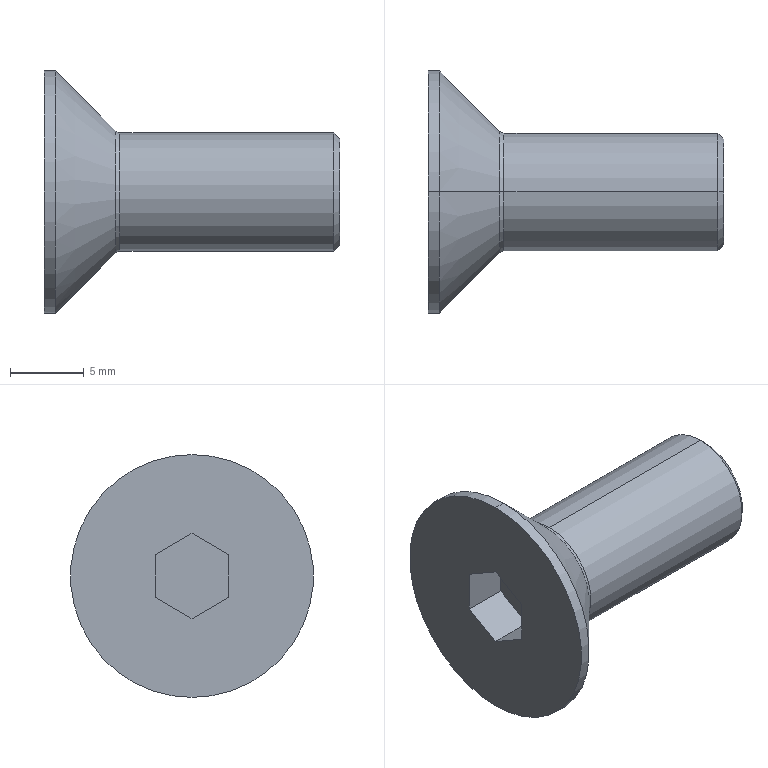Part | STEP file | 1 solid | 19 faces | box 20 x 16.428 x 16.428 mm | volume 1361 mm3 | plane 9 | cone 4 | cylinder 4 | spline 2 | commonest cylinder face diameters 8 x2 16.428 x2
STEP:
#1=CARTESIAN_POINT('',(0.,0.,0.));
#2=DIRECTION('',(0.,0.,1.));
#3=DIRECTION('',(1.,0.,0.));
#4=AXIS2_PLACEMENT_3D('',#1,#2,#3);
#5=CARTESIAN_POINT('',(15.04,0.,3.6));
#6=VERTEX_POINT('',#5);
#7=CARTESIAN_POINT('',(15.04,0.,-3.6));
#8=VERTEX_POINT('',#7);
#9=CARTESIAN_POINT('',(15.04,0.,0.));
#10=DIRECTION('',(-1.,0.,0.));
#11=DIRECTION('',(0.,0.,1.));
#12=AXIS2_PLACEMENT_3D('',#9,#10,#11);
#13=CIRCLE('',#12,3.6);
#14=CARTESIAN_POINT('',(15.04,4.,0.));
#15=DIRECTION('',(-1.,0.,0.));
#16=DIRECTION('',(0.,0.,1.));
#17=AXIS2_PLACEMENT_3D('',#14,#15,#16);
#18=PLANE('',#17);
#19=CARTESIAN_POINT('',(0.,-4.));
#20=DIRECTION('',(1.,0.));
#21=AXIS2_PLACEMENT_2D('',#19,#20);
#22=CIRCLE('',#21,3.6);
#23=(GEOMETRIC_REPRESENTATION_CONTEXT(2)PARAMETRIC_REPRESENTATION_CONTEXT()REPRESENTATION_CONTEXT('',''));
#24=DEFINITIONAL_REPRESENTATION('',(#22),#23);
#25=PCURVE('',#18,#24);
#26=CARTESIAN_POINT('',(14.64,0.,0.));
#27=DIRECTION('',(-1.,0.,0.));
#28=DIRECTION('',(0.,0.,1.));
#29=AXIS2_PLACEMENT_3D('',#26,#27,#28);
#30=CONICAL_SURFACE('',#29,4.,0.7854);
#31=CARTESIAN_POINT('',(0.,-0.4));
#32=DIRECTION('',(1.,0.));
#33=VECTOR('',#32,1.);
#34=LINE('',#31,#33);
#35=(GEOMETRIC_REPRESENTATION_CONTEXT(2)PARAMETRIC_REPRESENTATION_CONTEXT()REPRESENTATION_CONTEXT('',''));
#36=DEFINITIONAL_REPRESENTATION('',(#34),#35);
#37=PCURVE('',#30,#36);
#38=SURFACE_CURVE('',#13,(#25,#37),.PCURVE_S1.);
#39=EDGE_CURVE('',#6,#8,#38,.T.);
#40=ORIENTED_EDGE('',*,*,#39,.F.);
#41=CARTESIAN_POINT('',(15.04,0.,0.));
#42=DIRECTION('',(-1.,0.,0.));
#43=DIRECTION('',(0.,0.,1.));
#44=AXIS2_PLACEMENT_3D('',#41,#42,#43);
#45=CIRCLE('',#44,3.6);
#46=CARTESIAN_POINT('',(0.,-4.));
#47=DIRECTION('',(1.,0.));
#48=AXIS2_PLACEMENT_2D('',#46,#47);
#49=CIRCLE('',#48,3.6);
#50=(GEOMETRIC_REPRESENTATION_CONTEXT(2)PARAMETRIC_REPRESENTATION_CONTEXT()REPRESENTATION_CONTEXT('',''));
#51=DEFINITIONAL_REPRESENTATION('',(#49),#50);
#52=PCURVE('',#18,#51);
#53=CARTESIAN_POINT('',(14.64,0.,0.));
#54=DIRECTION('',(-1.,0.,0.));
#55=DIRECTION('',(0.,0.,1.));
#56=AXIS2_PLACEMENT_3D('',#53,#54,#55);
#57=CONICAL_SURFACE('',#56,4.,0.7854);
#58=CARTESIAN_POINT('',(0.,-0.4));
#59=DIRECTION('',(1.,0.));
#60=VECTOR('',#59,1.);
#61=LINE('',#58,#60);
#62=(GEOMETRIC_REPRESENTATION_CONTEXT(2)PARAMETRIC_REPRESENTATION_CONTEXT()REPRESENTATION_CONTEXT('',''));
#63=DEFINITIONAL_REPRESENTATION('',(#61),#62);
#64=PCURVE('',#57,#63);
#65=SURFACE_CURVE('',#45,(#52,#64),.PCURVE_S1.);
#66=EDGE_CURVE('',#8,#6,#65,.T.);
#67=ORIENTED_EDGE('',*,*,#66,.F.);
#68=EDGE_LOOP('',(#40,#67));
#69=FACE_BOUND('',#68,.T.);
#70=ADVANCED_FACE('',(#69),#18,.F.);
#71=CARTESIAN_POINT('',(14.64,0.,-4.));
#72=VERTEX_POINT('',#71);
#73=CARTESIAN_POINT('',(14.64,0.,-4.));
#74=DIRECTION('',(-0.7071,0.,-0.7071));
#75=VECTOR('',#74,1.);
#76=LINE('',#73,#75);
#77=CARTESIAN_POINT('',(3.142,0.));
#78=DIRECTION('',(0.,1.));
#79=VECTOR('',#78,1.);
#80=LINE('',#77,#79);
#81=(GEOMETRIC_REPRESENTATION_CONTEXT(2)PARAMETRIC_REPRESENTATION_CONTEXT()REPRESENTATION_CONTEXT('',''));
#82=DEFINITIONAL_REPRESENTATION('',(#80),#81);
#83=PCURVE('',#57,#82);
#84=CARTESIAN_POINT('',(3.142,0.));
#85=DIRECTION('',(0.,1.));
#86=VECTOR('',#85,1.);
#87=LINE('',#84,#86);
#88=(GEOMETRIC_REPRESENTATION_CONTEXT(2)PARAMETRIC_REPRESENTATION_CONTEXT()REPRESENTATION_CONTEXT('',''));
#89=DEFINITIONAL_REPRESENTATION('',(#87),#88);
#90=PCURVE('',#30,#89);
#91=SURFACE_CURVE('',#76,(#83,#90),.PCURVE_S1.);
#92=EDGE_CURVE('',#8,#72,#91,.T.);
#93=ORIENTED_EDGE('',*,*,#92,.F.);
#94=ORIENTED_EDGE('',*,*,#66,.T.);
#95=CARTESIAN_POINT('',(14.64,0.,4.));
#96=VERTEX_POINT('',#95);
#97=CARTESIAN_POINT('',(14.64,0.,4.));
#98=DIRECTION('',(-0.7071,0.,0.7071));
#99=VECTOR('',#98,1.);
#100=LINE('',#97,#99);
#101=CARTESIAN_POINT('',(6.283,0.));
#102=DIRECTION('',(0.,1.));
#103=VECTOR('',#102,1.);
#104=LINE('',#101,#103);
#105=(GEOMETRIC_REPRESENTATION_CONTEXT(2)PARAMETRIC_REPRESENTATION_CONTEXT()REPRESENTATION_CONTEXT('',''));
#106=DEFINITIONAL_REPRESENTATION('',(#104),#105);
#107=PCURVE('',#57,#106);
#108=CARTESIAN_POINT('',(0.,0.));
#109=DIRECTION('',(0.,1.));
#110=VECTOR('',#109,1.);
#111=LINE('',#108,#110);
#112=(GEOMETRIC_REPRESENTATION_CONTEXT(2)PARAMETRIC_REPRESENTATION_CONTEXT()REPRESENTATION_CONTEXT('',''));
#113=DEFINITIONAL_REPRESENTATION('',(#111),#112);
#114=PCURVE('',#30,#113);
#115=SURFACE_CURVE('',#100,(#107,#114),.PCURVE_S1.);
#116=EDGE_CURVE('',#6,#96,#115,.T.);
#117=ORIENTED_EDGE('',*,*,#116,.T.);
#118=CARTESIAN_POINT('',(14.64,0.,0.));
#119=DIRECTION('',(-1.,0.,0.));
#120=DIRECTION('',(0.,0.,1.));
#121=AXIS2_PLACEMENT_3D('',#118,#119,#120);
#122=CIRCLE('',#121,4.);
#123=CARTESIAN_POINT('',(0.,0.));
#124=DIRECTION('',(1.,0.));
#125=VECTOR('',#124,1.);
#126=LINE('',#123,#125);
#127=(GEOMETRIC_REPRESENTATION_CONTEXT(2)PARAMETRIC_REPRESENTATION_CONTEXT()REPRESENTATION_CONTEXT('',''));
#128=DEFINITIONAL_REPRESENTATION('',(#126),#127);
#129=PCURVE('',#57,#128);
#130=CARTESIAN_POINT('',(-23.423,0.,0.));
#131=DIRECTION('',(-1.,0.,0.));
#132=DIRECTION('',(0.,0.,1.));
#133=AXIS2_PLACEMENT_3D('',#130,#131,#132);
#134=CYLINDRICAL_SURFACE('',#133,4.);
#135=CARTESIAN_POINT('',(0.,-38.063));
#136=DIRECTION('',(1.,0.));
#137=VECTOR('',#136,1.);
#138=LINE('',#135,#137);
#139=(GEOMETRIC_REPRESENTATION_CONTEXT(2)PARAMETRIC_REPRESENTATION_CONTEXT()REPRESENTATION_CONTEXT('',''));
#140=DEFINITIONAL_REPRESENTATION('',(#138),#139);
#141=PCURVE('',#134,#140);
#142=SURFACE_CURVE('',#122,(#129,#141),.PCURVE_S1.);
#143=EDGE_CURVE('',#72,#96,#142,.T.);
#144=ORIENTED_EDGE('',*,*,#143,.F.);
#145=EDGE_LOOP('',(#93,#94,#117,#144));
#146=FACE_BOUND('',#145,.T.);
#147=ADVANCED_FACE('',(#146),#57,.T.);
#148=CARTESIAN_POINT('',(0.1657,0.,-4.));
#149=VERTEX_POINT('',#148);
#150=CARTESIAN_POINT('',(-23.423,0.,-4.));
#151=DIRECTION('',(-1.,0.,0.));
#152=VECTOR('',#151,1.);
#153=LINE('',#150,#152);
#154=CARTESIAN_POINT('',(3.142,0.));
#155=DIRECTION('',(0.,1.));
#156=VECTOR('',#155,1.);
#157=LINE('',#154,#156);
#158=(GEOMETRIC_REPRESENTATION_CONTEXT(2)PARAMETRIC_REPRESENTATION_CONTEXT()REPRESENTATION_CONTEXT('',''));
#159=DEFINITIONAL_REPRESENTATION('',(#157),#158);
#160=PCURVE('',#134,#159);
#161=CARTESIAN_POINT('',(-23.423,0.,0.));
#162=DIRECTION('',(-1.,0.,0.));
#163=DIRECTION('',(0.,0.,1.));
#164=AXIS2_PLACEMENT_3D('',#161,#162,#163);
#165=CYLINDRICAL_SURFACE('',#164,4.);
#166=CARTESIAN_POINT('',(3.142,0.));
#167=DIRECTION('',(0.,1.));
#168=VECTOR('',#167,1.);
#169=LINE('',#166,#168);
#170=(GEOMETRIC_REPRESENTATION_CONTEXT(2)PARAMETRIC_REPRESENTATION_CONTEXT()REPRESENTATION_CONTEXT('',''));
#171=DEFINITIONAL_REPRESENTATION('',(#169),#170);
#172=PCURVE('',#165,#171);
#173=SURFACE_CURVE('',#153,(#160,#172),.PCURVE_S1.);
#174=EDGE_CURVE('',#72,#149,#173,.T.);
#175=ORIENTED_EDGE('',*,*,#174,.F.);
#176=ORIENTED_EDGE('',*,*,#143,.T.);
#177=CARTESIAN_POINT('',(0.1657,0.,4.));
#178=VERTEX_POINT('',#177);
#179=CARTESIAN_POINT('',(-23.423,0.,4.));
#180=DIRECTION('',(-1.,0.,0.));
#181=VECTOR('',#180,1.);
#182=LINE('',#179,#181);
#183=CARTESIAN_POINT('',(6.283,0.));
#184=DIRECTION('',(0.,1.));
#185=VECTOR('',#184,1.);
#186=LINE('',#183,#185);
#187=(GEOMETRIC_REPRESENTATION_CONTEXT(2)PARAMETRIC_REPRESENTATION_CONTEXT()REPRESENTATION_CONTEXT('',''));
#188=DEFINITIONAL_REPRESENTATION('',(#186),#187);
#189=PCURVE('',#134,#188);
#190=CARTESIAN_POINT('',(0.,0.));
#191=DIRECTION('',(0.,1.));
#192=VECTOR('',#191,1.);
#193=LINE('',#190,#192);
#194=(GEOMETRIC_REPRESENTATION_CONTEXT(2)PARAMETRIC_REPRESENTATION_CONTEXT()REPRESENTATION_CONTEXT('',''));
#195=DEFINITIONAL_REPRESENTATION('',(#193),#194);
#196=PCURVE('',#165,#195);
#197=SURFACE_CURVE('',#182,(#189,#196),.PCURVE_S1.);
#198=EDGE_CURVE('',#96,#178,#197,.T.);
#199=ORIENTED_EDGE('',*,*,#198,.T.);
#200=CARTESIAN_POINT('',(0.1657,0.,0.));
#201=DIRECTION('',(1.,0.,0.));
#202=DIRECTION('',(0.,0.,1.));
#203=AXIS2_PLACEMENT_3D('',#200,#201,#202);
#204=CIRCLE('',#203,4.);
#205=CARTESIAN_POINT('',(6.283,-23.589));
#206=DIRECTION('',(-1.,0.));
#207=VECTOR('',#206,1.);
#208=LINE('',#205,#207);
#209=(GEOMETRIC_REPRESENTATION_CONTEXT(2)PARAMETRIC_REPRESENTATION_CONTEXT()REPRESENTATION_CONTEXT('',''));
#210=DEFINITIONAL_REPRESENTATION('',(#208),#209);
#211=PCURVE('',#134,#210);
#212=CARTESIAN_POINT('',(0.1657,0.,-4.));
#213=CARTESIAN_POINT('',(0.1657,-8.,-4.));
#214=CARTESIAN_POINT('',(0.1657,-8.,4.));
#215=CARTESIAN_POINT('',(0.1657,0.,4.));
#216=CARTESIAN_POINT('',(0.05818,0.,-4.));
#217=CARTESIAN_POINT('',(0.05818,-8.,-4.));
#218=CARTESIAN_POINT('',(0.05818,-8.,4.));
#219=CARTESIAN_POINT('',(0.05818,0.,4.));
#220=CARTESIAN_POINT('',(-0.04114,0.,-4.041));
#221=CARTESIAN_POINT('',(-0.04114,-8.082,-4.041));
#222=CARTESIAN_POINT('',(-0.04114,-8.082,4.041));
#223=CARTESIAN_POINT('',(-0.04114,0.,4.041));
#224=CARTESIAN_POINT('',(-0.1172,0.,-4.117));
#225=CARTESIAN_POINT('',(-0.1172,-8.234,-4.117));
#226=CARTESIAN_POINT('',(-0.1172,-8.234,4.117));
#227=CARTESIAN_POINT('',(-0.1172,0.,4.117));
#228=(BOUNDED_SURFACE()B_SPLINE_SURFACE(3,3,((#212,#213,#214,#215),(#216,#217,#218,#219),(#220,#221,#222,#223),(#224,#225,#226,#227)),.UNSPECIFIED.,.F.,.F.,.F.)B_SPLINE_SURFACE_WITH_KNOTS((4,4),(4,4),(0.,1.),(0.,1.),.PIECEWISE_BEZIER_KNOTS.)GEOMETRIC_REPRESENTATION_ITEM()RATIONAL_B_SPLINE_SURFACE(((1.,0.3333,0.3333,1.),(0.9493,0.3164,0.3164,0.9493),(0.9493,0.3164,0.3164,0.9493),(1.,0.3333,0.3333,1.)))REPRESENTATION_ITEM('')SURFACE());
#229=CARTESIAN_POINT('',(0.,1.));
#230=CARTESIAN_POINT('',(0.,0.9763));
#231=CARTESIAN_POINT('',(0.,0.9319));
#232=CARTESIAN_POINT('',(0.,0.8733));
#233=CARTESIAN_POINT('',(0.,0.8206));
#234=CARTESIAN_POINT('',(0.,0.7724));
#235=CARTESIAN_POINT('',(0.,0.7279));
#236=CARTESIAN_POINT('',(0.,0.6861));
#237=CARTESIAN_POINT('',(0.,0.6465));
#238=CARTESIAN_POINT('',(0.,0.6086));
#239=CARTESIAN_POINT('',(0.,0.5718));
#240=CARTESIAN_POINT('',(0.,0.5357));
#241=CARTESIAN_POINT('',(0.,0.5));
#242=CARTESIAN_POINT('',(0.,0.4643));
#243=CARTESIAN_POINT('',(0.,0.4282));
#244=CARTESIAN_POINT('',(0.,0.3914));
#245=CARTESIAN_POINT('',(0.,0.3535));
#246=CARTESIAN_POINT('',(0.,0.3139));
#247=CARTESIAN_POINT('',(0.,0.2721));
#248=CARTESIAN_POINT('',(0.,0.2276));
#249=CARTESIAN_POINT('',(0.,0.1794));
#250=CARTESIAN_POINT('',(0.,0.1267));
#251=CARTESIAN_POINT('',(0.,0.06805));
#252=CARTESIAN_POINT('',(0.,0.02375));
#253=CARTESIAN_POINT('',(0.,0.));
#254=B_SPLINE_CURVE_WITH_KNOTS('',3,(#229,#230,#231,#232,#233,#234,#235,#236,#237,#238,#239,#240,#241,#242,#243,#244,#245,#246,#247,#248,#249,#250,#251,#252,#253),.UNSPECIFIED.,.F.,.F.,(4,1,1,1,1,1,1,1,1,1,1,1,1,1,1,1,1,1,1,1,1,1,4),(0.,0.1428,0.2856,0.4284,0.5712,0.714,0.8568,0.9996,1.142,1.285,1.428,1.571,1.714,1.856,1.999,2.142,2.285,2.428,2.57,2.713,2.856,2.999,3.142),.QUASI_UNIFORM_KNOTS.);
#255=(GEOMETRIC_REPRESENTATION_CONTEXT(2)PARAMETRIC_REPRESENTATION_CONTEXT()REPRESENTATION_CONTEXT('',''));
#256=DEFINITIONAL_REPRESENTATION('',(#254),#255);
#257=PCURVE('',#228,#256);
#258=SURFACE_CURVE('',#204,(#211,#257),.PCURVE_S1.);
#259=EDGE_CURVE('',#178,#149,#258,.T.);
#260=ORIENTED_EDGE('',*,*,#259,.T.);
#261=EDGE_LOOP('',(#175,#176,#199,#260));
#262=FACE_BOUND('',#261,.T.);
#263=ADVANCED_FACE('',(#262),#134,.T.);
#264=CARTESIAN_POINT('',(-0.1172,0.,-4.117));
#265=VERTEX_POINT('',#264);
#266=CARTESIAN_POINT('',(-0.1172,0.,4.117));
#267=VERTEX_POINT('',#266);
#268=CARTESIAN_POINT('',(-0.1172,0.,0.));
#269=DIRECTION('',(-1.,0.,0.));
#270=DIRECTION('',(0.,0.,1.));
#271=AXIS2_PLACEMENT_3D('',#268,#269,#270);
#272=CIRCLE('',#271,4.117);
#273=CARTESIAN_POINT('',(1.,0.));
#274=CARTESIAN_POINT('',(1.,0.02375));
#275=CARTESIAN_POINT('',(1.,0.06805));
#276=CARTESIAN_POINT('',(1.,0.1267));
#277=CARTESIAN_POINT('',(1.,0.1794));
#278=CARTESIAN_POINT('',(1.,0.2276));
#279=CARTESIAN_POINT('',(1.,0.2721));
#280=CARTESIAN_POINT('',(1.,0.3139));
#281=CARTESIAN_POINT('',(1.,0.3535));
#282=CARTESIAN_POINT('',(1.,0.3914));
#283=CARTESIAN_POINT('',(1.,0.4282));
#284=CARTESIAN_POINT('',(1.,0.4643));
#285=CARTESIAN_POINT('',(1.,0.5));
#286=CARTESIAN_POINT('',(1.,0.5357));
#287=CARTESIAN_POINT('',(1.,0.5718));
#288=CARTESIAN_POINT('',(1.,0.6086));
#289=CARTESIAN_POINT('',(1.,0.6465));
#290=CARTESIAN_POINT('',(1.,0.6861));
#291=CARTESIAN_POINT('',(1.,0.7279));
#292=CARTESIAN_POINT('',(1.,0.7724));
#293=CARTESIAN_POINT('',(1.,0.8206));
#294=CARTESIAN_POINT('',(1.,0.8733));
#295=CARTESIAN_POINT('',(1.,0.9319));
#296=CARTESIAN_POINT('',(1.,0.9763));
#297=CARTESIAN_POINT('',(1.,1.));
#298=B_SPLINE_CURVE_WITH_KNOTS('',3,(#273,#274,#275,#276,#277,#278,#279,#280,#281,#282,#283,#284,#285,#286,#287,#288,#289,#290,#291,#292,#293,#294,#295,#296,#297),.UNSPECIFIED.,.F.,.F.,(4,1,1,1,1,1,1,1,1,1,1,1,1,1,1,1,1,1,1,1,1,1,4),(3.142,3.284,3.427,3.57,3.713,3.856,3.998,4.141,4.284,4.427,4.57,4.712,4.855,4.998,5.141,5.284,5.426,5.569,5.712,5.855,5.998,6.14,6.283),.QUASI_UNIFORM_KNOTS.);
#299=(GEOMETRIC_REPRESENTATION_CONTEXT(2)PARAMETRIC_REPRESENTATION_CONTEXT()REPRESENTATION_CONTEXT('',''));
#300=DEFINITIONAL_REPRESENTATION('',(#298),#299);
#301=PCURVE('',#228,#300);
#302=CARTESIAN_POINT('',(-4.214,0.,0.));
#303=DIRECTION('',(-1.,0.,0.));
#304=DIRECTION('',(0.,0.,1.));
#305=AXIS2_PLACEMENT_3D('',#302,#303,#304);
#306=CONICAL_SURFACE('',#305,8.214,0.7854);
#307=CARTESIAN_POINT('',(0.,-4.097));
#308=DIRECTION('',(1.,0.));
#309=VECTOR('',#308,1.);
#310=LINE('',#307,#309);
#311=(GEOMETRIC_REPRESENTATION_CONTEXT(2)PARAMETRIC_REPRESENTATION_CONTEXT()REPRESENTATION_CONTEXT('',''));
#312=DEFINITIONAL_REPRESENTATION('',(#310),#311);
#313=PCURVE('',#306,#312);
#314=SURFACE_CURVE('',#272,(#301,#313),.PCURVE_S1.);
#315=EDGE_CURVE('',#265,#267,#314,.T.);
#316=ORIENTED_EDGE('',*,*,#315,.T.);
#317=CARTESIAN_POINT('',(0.1657,0.,4.4));
#318=DIRECTION('',(0.,1.,0.));
#319=DIRECTION('',(0.,0.,1.));
#320=AXIS2_PLACEMENT_3D('',#317,#318,#319);
#321=CIRCLE('',#320,0.4);
#322=CARTESIAN_POINT('',(0.,1.));
#323=CARTESIAN_POINT('',(0.01555,1.));
#324=CARTESIAN_POINT('',(0.04653,1.));
#325=CARTESIAN_POINT('',(0.09271,1.));
#326=CARTESIAN_POINT('',(0.1386,1.));
#327=CARTESIAN_POINT('',(0.1843,1.));
#328=CARTESIAN_POINT('',(0.2298,1.));
#329=CARTESIAN_POINT('',(0.2751,1.));
#330=CARTESIAN_POINT('',(0.3202,1.));
#331=CARTESIAN_POINT('',(0.3653,1.));
#332=CARTESIAN_POINT('',(0.4102,1.));
#333=CARTESIAN_POINT('',(0.4551,1.));
#334=CARTESIAN_POINT('',(0.5,1.));
#335=CARTESIAN_POINT('',(0.5449,1.));
#336=CARTESIAN_POINT('',(0.5898,1.));
#337=CARTESIAN_POINT('',(0.6347,1.));
#338=CARTESIAN_POINT('',(0.6798,1.));
#339=CARTESIAN_POINT('',(0.7249,1.));
#340=CARTESIAN_POINT('',(0.7702,1.));
#341=CARTESIAN_POINT('',(0.8157,1.));
#342=CARTESIAN_POINT('',(0.8614,1.));
#343=CARTESIAN_POINT('',(0.9073,1.));
#344=CARTESIAN_POINT('',(0.9535,1.));
#345=CARTESIAN_POINT('',(0.9845,1.));
#346=CARTESIAN_POINT('',(1.,1.));
#347=B_SPLINE_CURVE_WITH_KNOTS('',3,(#322,#323,#324,#325,#326,#327,#328,#329,#330,#331,#332,#333,#334,#335,#336,#337,#338,#339,#340,#341,#342,#343,#344,#345,#346),.UNSPECIFIED.,.F.,.F.,(4,1,1,1,1,1,1,1,1,1,1,1,1,1,1,1,1,1,1,1,1,1,4),(3.142,3.177,3.213,3.249,3.284,3.32,3.356,3.391,3.427,3.463,3.499,3.534,3.57,3.606,3.641,3.677,3.713,3.748,3.784,3.82,3.856,3.891,3.927),.QUASI_UNIFORM_KNOTS.);
#348=(GEOMETRIC_REPRESENTATION_CONTEXT(2)PARAMETRIC_REPRESENTATION_CONTEXT()REPRESENTATION_CONTEXT('',''));
#349=DEFINITIONAL_REPRESENTATION('',(#347),#348);
#350=PCURVE('',#228,#349);
#351=CARTESIAN_POINT('',(0.1657,0.,4.));
#352=CARTESIAN_POINT('',(0.1657,8.,4.));
#353=CARTESIAN_POINT('',(0.1657,8.,-4.));
#354=CARTESIAN_POINT('',(0.1657,0.,-4.));
#355=CARTESIAN_POINT('',(0.05818,0.,4.));
#356=CARTESIAN_POINT('',(0.05818,8.,4.));
#357=CARTESIAN_POINT('',(0.05818,8.,-4.));
#358=CARTESIAN_POINT('',(0.05818,0.,-4.));
#359=CARTESIAN_POINT('',(-0.04114,0.,4.041));
#360=CARTESIAN_POINT('',(-0.04114,8.082,4.041));
#361=CARTESIAN_POINT('',(-0.04114,8.082,-4.041));
#362=CARTESIAN_POINT('',(-0.04114,0.,-4.041));
#363=CARTESIAN_POINT('',(-0.1172,0.,4.117));
#364=CARTESIAN_POINT('',(-0.1172,8.234,4.117));
#365=CARTESIAN_POINT('',(-0.1172,8.234,-4.117));
#366=CARTESIAN_POINT('',(-0.1172,0.,-4.117));
#367=(BOUNDED_SURFACE()B_SPLINE_SURFACE(3,3,((#351,#352,#353,#354),(#355,#356,#357,#358),(#359,#360,#361,#362),(#363,#364,#365,#366)),.UNSPECIFIED.,.F.,.F.,.F.)B_SPLINE_SURFACE_WITH_KNOTS((4,4),(4,4),(0.,1.),(0.,1.),.PIECEWISE_BEZIER_KNOTS.)GEOMETRIC_REPRESENTATION_ITEM()RATIONAL_B_SPLINE_SURFACE(((1.,0.3333,0.3333,1.),(0.9493,0.3164,0.3164,0.9493),(0.9493,0.3164,0.3164,0.9493),(1.,0.3333,0.3333,1.)))REPRESENTATION_ITEM('')SURFACE());
#368=CARTESIAN_POINT('',(0.,0.));
#369=CARTESIAN_POINT('',(0.01555,0.));
#370=CARTESIAN_POINT('',(0.04653,0.));
#371=CARTESIAN_POINT('',(0.09271,0.));
#372=CARTESIAN_POINT('',(0.1386,0.));
#373=CARTESIAN_POINT('',(0.1843,0.));
#374=CARTESIAN_POINT('',(0.2298,0.));
#375=CARTESIAN_POINT('',(0.2751,0.));
#376=CARTESIAN_POINT('',(0.3202,0.));
#377=CARTESIAN_POINT('',(0.3653,0.));
#378=CARTESIAN_POINT('',(0.4102,0.));
#379=CARTESIAN_POINT('',(0.4551,0.));
#380=CARTESIAN_POINT('',(0.5,0.));
#381=CARTESIAN_POINT('',(0.5449,0.));
#382=CARTESIAN_POINT('',(0.5898,0.));
#383=CARTESIAN_POINT('',(0.6347,0.));
#384=CARTESIAN_POINT('',(0.6798,0.));
#385=CARTESIAN_POINT('',(0.7249,0.));
#386=CARTESIAN_POINT('',(0.7702,0.));
#387=CARTESIAN_POINT('',(0.8157,0.));
#388=CARTESIAN_POINT('',(0.8614,0.));
#389=CARTESIAN_POINT('',(0.9073,0.));
#390=CARTESIAN_POINT('',(0.9535,0.));
#391=CARTESIAN_POINT('',(0.9845,0.));
#392=CARTESIAN_POINT('',(1.,0.));
#393=B_SPLINE_CURVE_WITH_KNOTS('',3,(#368,#369,#370,#371,#372,#373,#374,#375,#376,#377,#378,#379,#380,#381,#382,#383,#384,#385,#386,#387,#388,#389,#390,#391,#392),.UNSPECIFIED.,.F.,.F.,(4,1,1,1,1,1,1,1,1,1,1,1,1,1,1,1,1,1,1,1,1,1,4),(3.142,3.177,3.213,3.249,3.284,3.32,3.356,3.391,3.427,3.463,3.499,3.534,3.57,3.606,3.641,3.677,3.713,3.748,3.784,3.82,3.856,3.891,3.927),.QUASI_UNIFORM_KNOTS.);
#394=(GEOMETRIC_REPRESENTATION_CONTEXT(2)PARAMETRIC_REPRESENTATION_CONTEXT()REPRESENTATION_CONTEXT('',''));
#395=DEFINITIONAL_REPRESENTATION('',(#393),#394);
#396=PCURVE('',#367,#395);
#397=SURFACE_CURVE('',#321,(#350,#396),.PCURVE_S1.);
#398=EDGE_CURVE('',#178,#267,#397,.T.);
#399=ORIENTED_EDGE('',*,*,#398,.F.);
#400=ORIENTED_EDGE('',*,*,#259,.T.);
#401=CARTESIAN_POINT('',(0.1657,0.,-4.4));
#402=DIRECTION('',(0.,-1.,0.));
#403=DIRECTION('',(0.,0.,-1.));
#404=AXIS2_PLACEMENT_3D('',#401,#402,#403);
#405=CIRCLE('',#404,0.4);
#406=CARTESIAN_POINT('',(0.,0.));
#407=CARTESIAN_POINT('',(0.01555,0.));
#408=CARTESIAN_POINT('',(0.04653,0.));
#409=CARTESIAN_POINT('',(0.09271,0.));
#410=CARTESIAN_POINT('',(0.1386,0.));
#411=CARTESIAN_POINT('',(0.1843,0.));
#412=CARTESIAN_POINT('',(0.2298,0.));
#413=CARTESIAN_POINT('',(0.2751,0.));
#414=CARTESIAN_POINT('',(0.3202,0.));
#415=CARTESIAN_POINT('',(0.3653,0.));
#416=CARTESIAN_POINT('',(0.4102,0.));
#417=CARTESIAN_POINT('',(0.4551,0.));
#418=CARTESIAN_POINT('',(0.5,0.));
#419=CARTESIAN_POINT('',(0.5449,0.));
#420=CARTESIAN_POINT('',(0.5898,0.));
#421=CARTESIAN_POINT('',(0.6347,0.));
#422=CARTESIAN_POINT('',(0.6798,0.));
#423=CARTESIAN_POINT('',(0.7249,0.));
#424=CARTESIAN_POINT('',(0.7702,0.));
#425=CARTESIAN_POINT('',(0.8157,0.));
#426=CARTESIAN_POINT('',(0.8614,0.));
#427=CARTESIAN_POINT('',(0.9073,0.));
#428=CARTESIAN_POINT('',(0.9535,0.));
#429=CARTESIAN_POINT('',(0.9845,0.));
#430=CARTESIAN_POINT('',(1.,0.));
#431=B_SPLINE_CURVE_WITH_KNOTS('',3,(#406,#407,#408,#409,#410,#411,#412,#413,#414,#415,#416,#417,#418,#419,#420,#421,#422,#423,#424,#425,#426,#427,#428,#429,#430),.UNSPECIFIED.,.F.,.F.,(4,1,1,1,1,1,1,1,1,1,1,1,1,1,1,1,1,1,1,1,1,1,4),(3.142,3.177,3.213,3.249,3.284,3.32,3.356,3.391,3.427,3.463,3.499,3.534,3.57,3.606,3.641,3.677,3.713,3.748,3.784,3.82,3.856,3.891,3.927),.QUASI_UNIFORM_KNOTS.);
#432=(GEOMETRIC_REPRESENTATION_CONTEXT(2)PARAMETRIC_REPRESENTATION_CONTEXT()REPRESENTATION_CONTEXT('',''));
#433=DEFINITIONAL_REPRESENTATION('',(#431),#432);
#434=PCURVE('',#228,#433);
#435=CARTESIAN_POINT('',(0.,1.));
#436=CARTESIAN_POINT('',(0.01555,1.));
#437=CARTESIAN_POINT('',(0.04653,1.));
#438=CARTESIAN_POINT('',(0.09271,1.));
#439=CARTESIAN_POINT('',(0.1386,1.));
#440=CARTESIAN_POINT('',(0.1843,1.));
#441=CARTESIAN_POINT('',(0.2298,1.));
#442=CARTESIAN_POINT('',(0.2751,1.));
#443=CARTESIAN_POINT('',(0.3202,1.));
#444=CARTESIAN_POINT('',(0.3653,1.));
#445=CARTESIAN_POINT('',(0.4102,1.));
#446=CARTESIAN_POINT('',(0.4551,1.));
#447=CARTESIAN_POINT('',(0.5,1.));
#448=CARTESIAN_POINT('',(0.5449,1.));
#449=CARTESIAN_POINT('',(0.5898,1.));
#450=CARTESIAN_POINT('',(0.6347,1.));
#451=CARTESIAN_POINT('',(0.6798,1.));
#452=CARTESIAN_POINT('',(0.7249,1.));
#453=CARTESIAN_POINT('',(0.7702,1.));
#454=CARTESIAN_POINT('',(0.8157,1.));
#455=CARTESIAN_POINT('',(0.8614,1.));
#456=CARTESIAN_POINT('',(0.9073,1.));
#457=CARTESIAN_POINT('',(0.9535,1.));
#458=CARTESIAN_POINT('',(0.9845,1.));
#459=CARTESIAN_POINT('',(1.,1.));
#460=B_SPLINE_CURVE_WITH_KNOTS('',3,(#435,#436,#437,#438,#439,#440,#441,#442,#443,#444,#445,#446,#447,#448,#449,#450,#451,#452,#453,#454,#455,#456,#457,#458,#459),.UNSPECIFIED.,.F.,.F.,(4,1,1,1,1,1,1,1,1,1,1,1,1,1,1,1,1,1,1,1,1,1,4),(3.142,3.177,3.213,3.249,3.284,3.32,3.356,3.391,3.427,3.463,3.499,3.534,3.57,3.606,3.641,3.677,3.713,3.748,3.784,3.82,3.856,3.891,3.927),.QUASI_UNIFORM_KNOTS.);
#461=(GEOMETRIC_REPRESENTATION_CONTEXT(2)PARAMETRIC_REPRESENTATION_CONTEXT()REPRESENTATION_CONTEXT('',''));
#462=DEFINITIONAL_REPRESENTATION('',(#460),#461);
#463=PCURVE('',#367,#462);
#464=SURFACE_CURVE('',#405,(#434,#463),.PCURVE_S1.);
#465=EDGE_CURVE('',#149,#265,#464,.T.);
#466=ORIENTED_EDGE('',*,*,#465,.T.);
#467=EDGE_LOOP('',(#316,#399,#400,#466));
#468=FACE_BOUND('',#467,.F.);
#469=ADVANCED_FACE('',(#468),#228,.F.);
#470=CARTESIAN_POINT('',(-1.96,-2.5,-1.443));
#471=VERTEX_POINT('',#470);
#472=CARTESIAN_POINT('',(-1.96,-2.5,1.443));
#473=VERTEX_POINT('',#472);
#474=CARTESIAN_POINT('',(-1.96,-2.5,-1.443));
#475=DIRECTION('',(0.,0.,1.));
#476=VECTOR('',#475,1.);
#477=LINE('',#474,#476);
#478=CARTESIAN_POINT('',(-1.96,0.,0.));
#479=DIRECTION('',(-1.,0.,0.));
#480=DIRECTION('',(0.,0.,1.));
#481=AXIS2_PLACEMENT_3D('',#478,#479,#480);
#482=PLANE('',#481);
#483=CARTESIAN_POINT('',(-1.443,-2.5));
#484=DIRECTION('',(1.,0.));
#485=VECTOR('',#484,1.);
#486=LINE('',#483,#485);
#487=(GEOMETRIC_REPRESENTATION_CONTEXT(2)PARAMETRIC_REPRESENTATION_CONTEXT()REPRESENTATION_CONTEXT('',''));
#488=DEFINITIONAL_REPRESENTATION('',(#486),#487);
#489=PCURVE('',#482,#488);
#490=CARTESIAN_POINT('',(-1.96,-2.5,-1.443));
#491=DIRECTION('',(0.,-1.,0.));
#492=DIRECTION('',(-1.,0.,0.));
#493=AXIS2_PLACEMENT_3D('',#490,#491,#492);
#494=PLANE('',#493);
#495=CARTESIAN_POINT('',(0.,0.));
#496=DIRECTION('',(0.,-1.));
#497=VECTOR('',#496,1.);
#498=LINE('',#495,#497);
#499=(GEOMETRIC_REPRESENTATION_CONTEXT(2)PARAMETRIC_REPRESENTATION_CONTEXT()REPRESENTATION_CONTEXT('',''));
#500=DEFINITIONAL_REPRESENTATION('',(#498),#499);
#501=PCURVE('',#494,#500);
#502=SURFACE_CURVE('',#477,(#489,#501),.PCURVE_S1.);
#503=EDGE_CURVE('',#471,#473,#502,.T.);
#504=ORIENTED_EDGE('',*,*,#503,.T.);
#505=CARTESIAN_POINT('',(-1.96,0.,2.887));
#506=VERTEX_POINT('',#505);
#507=CARTESIAN_POINT('',(-1.96,-2.5,1.443));
#508=DIRECTION('',(0.,0.866,0.5));
#509=VECTOR('',#508,1.);
#510=LINE('',#507,#509);
#511=CARTESIAN_POINT('',(1.443,-2.5));
#512=DIRECTION('',(0.5,0.866));
#513=VECTOR('',#512,1.);
#514=LINE('',#511,#513);
#515=(GEOMETRIC_REPRESENTATION_CONTEXT(2)PARAMETRIC_REPRESENTATION_CONTEXT()REPRESENTATION_CONTEXT('',''));
#516=DEFINITIONAL_REPRESENTATION('',(#514),#515);
#517=PCURVE('',#482,#516);
#518=CARTESIAN_POINT('',(-1.96,-2.5,1.443));
#519=DIRECTION('',(0.,-0.5,0.866));
#520=DIRECTION('',(-1.,0.,0.));
#521=AXIS2_PLACEMENT_3D('',#518,#519,#520);
#522=PLANE('',#521);
#523=CARTESIAN_POINT('',(0.,0.));
#524=DIRECTION('',(0.,-1.));
#525=VECTOR('',#524,1.);
#526=LINE('',#523,#525);
#527=(GEOMETRIC_REPRESENTATION_CONTEXT(2)PARAMETRIC_REPRESENTATION_CONTEXT()REPRESENTATION_CONTEXT('',''));
#528=DEFINITIONAL_REPRESENTATION('',(#526),#527);
#529=PCURVE('',#522,#528);
#530=SURFACE_CURVE('',#510,(#517,#529),.PCURVE_S1.);
#531=EDGE_CURVE('',#473,#506,#530,.T.);
#532=ORIENTED_EDGE('',*,*,#531,.T.);
#533=CARTESIAN_POINT('',(-1.96,2.5,1.443));
#534=VERTEX_POINT('',#533);
#535=CARTESIAN_POINT('',(-1.96,0.,2.887));
#536=DIRECTION('',(0.,0.866,-0.5));
#537=VECTOR('',#536,1.);
#538=LINE('',#535,#537);
#539=CARTESIAN_POINT('',(2.887,0.));
#540=DIRECTION('',(-0.5,0.866));
#541=VECTOR('',#540,1.);
#542=LINE('',#539,#541);
#543=(GEOMETRIC_REPRESENTATION_CONTEXT(2)PARAMETRIC_REPRESENTATION_CONTEXT()REPRESENTATION_CONTEXT('',''));
#544=DEFINITIONAL_REPRESENTATION('',(#542),#543);
#545=PCURVE('',#482,#544);
#546=CARTESIAN_POINT('',(-1.96,0.,2.887));
#547=DIRECTION('',(0.,0.5,0.866));
#548=DIRECTION('',(1.,0.,0.));
#549=AXIS2_PLACEMENT_3D('',#546,#547,#548);
#550=PLANE('',#549);
#551=CARTESIAN_POINT('',(0.,0.));
#552=DIRECTION('',(0.,1.));
#553=VECTOR('',#552,1.);
#554=LINE('',#551,#553);
#555=(GEOMETRIC_REPRESENTATION_CONTEXT(2)PARAMETRIC_REPRESENTATION_CONTEXT()REPRESENTATION_CONTEXT('',''));
#556=DEFINITIONAL_REPRESENTATION('',(#554),#555);
#557=PCURVE('',#550,#556);
#558=SURFACE_CURVE('',#538,(#545,#557),.PCURVE_S1.);
#559=EDGE_CURVE('',#506,#534,#558,.T.);
#560=ORIENTED_EDGE('',*,*,#559,.T.);
#561=CARTESIAN_POINT('',(-1.96,2.5,-1.443));
#562=VERTEX_POINT('',#561);
#563=CARTESIAN_POINT('',(-1.96,2.5,1.443));
#564=DIRECTION('',(0.,0.,-1.));
#565=VECTOR('',#564,1.);
#566=LINE('',#563,#565);
#567=CARTESIAN_POINT('',(1.443,2.5));
#568=DIRECTION('',(-1.,0.));
#569=VECTOR('',#568,1.);
#570=LINE('',#567,#569);
#571=(GEOMETRIC_REPRESENTATION_CONTEXT(2)PARAMETRIC_REPRESENTATION_CONTEXT()REPRESENTATION_CONTEXT('',''));
#572=DEFINITIONAL_REPRESENTATION('',(#570),#571);
#573=PCURVE('',#482,#572);
#574=CARTESIAN_POINT('',(-1.96,2.5,1.443));
#575=DIRECTION('',(0.,1.,0.));
#576=DIRECTION('',(0.,0.,-1.));
#577=AXIS2_PLACEMENT_3D('',#574,#575,#576);
#578=PLANE('',#577);
#579=CARTESIAN_POINT('',(0.,0.));
#580=DIRECTION('',(1.,0.));
#581=VECTOR('',#580,1.);
#582=LINE('',#579,#581);
#583=(GEOMETRIC_REPRESENTATION_CONTEXT(2)PARAMETRIC_REPRESENTATION_CONTEXT()REPRESENTATION_CONTEXT('',''));
#584=DEFINITIONAL_REPRESENTATION('',(#582),#583);
#585=PCURVE('',#578,#584);
#586=SURFACE_CURVE('',#566,(#573,#585),.PCURVE_S1.);
#587=EDGE_CURVE('',#534,#562,#586,.T.);
#588=ORIENTED_EDGE('',*,*,#587,.T.);
#589=CARTESIAN_POINT('',(-1.96,0.,-2.887));
#590=VERTEX_POINT('',#589);
#591=CARTESIAN_POINT('',(-1.96,2.5,-1.443));
#592=DIRECTION('',(0.,-0.866,-0.5));
#593=VECTOR('',#592,1.);
#594=LINE('',#591,#593);
#595=CARTESIAN_POINT('',(-1.443,2.5));
#596=DIRECTION('',(-0.5,-0.866));
#597=VECTOR('',#596,1.);
#598=LINE('',#595,#597);
#599=(GEOMETRIC_REPRESENTATION_CONTEXT(2)PARAMETRIC_REPRESENTATION_CONTEXT()REPRESENTATION_CONTEXT('',''));
#600=DEFINITIONAL_REPRESENTATION('',(#598),#599);
#601=PCURVE('',#482,#600);
#602=CARTESIAN_POINT('',(-1.96,2.5,-1.443));
#603=DIRECTION('',(0.,0.5,-0.866));
#604=DIRECTION('',(-1.,0.,0.));
#605=AXIS2_PLACEMENT_3D('',#602,#603,#604);
#606=PLANE('',#605);
#607=CARTESIAN_POINT('',(0.,0.));
#608=DIRECTION('',(0.,-1.));
#609=VECTOR('',#608,1.);
#610=LINE('',#607,#609);
#611=(GEOMETRIC_REPRESENTATION_CONTEXT(2)PARAMETRIC_REPRESENTATION_CONTEXT()REPRESENTATION_CONTEXT('',''));
#612=DEFINITIONAL_REPRESENTATION('',(#610),#611);
#613=PCURVE('',#606,#612);
#614=SURFACE_CURVE('',#594,(#601,#613),.PCURVE_S1.);
#615=EDGE_CURVE('',#562,#590,#614,.T.);
#616=ORIENTED_EDGE('',*,*,#615,.T.);
#617=CARTESIAN_POINT('',(-1.96,0.,-2.887));
#618=DIRECTION('',(0.,-0.866,0.5));
#619=VECTOR('',#618,1.);
#620=LINE('',#617,#619);
#621=CARTESIAN_POINT('',(-2.887,0.));
#622=DIRECTION('',(0.5,-0.866));
#623=VECTOR('',#622,1.);
#624=LINE('',#621,#623);
#625=(GEOMETRIC_REPRESENTATION_CONTEXT(2)PARAMETRIC_REPRESENTATION_CONTEXT()REPRESENTATION_CONTEXT('',''));
#626=DEFINITIONAL_REPRESENTATION('',(#624),#625);
#627=PCURVE('',#482,#626);
#628=CARTESIAN_POINT('',(-1.96,0.,-2.887));
#629=DIRECTION('',(0.,-0.5,-0.866));
#630=DIRECTION('',(0.,-0.866,0.5));
#631=AXIS2_PLACEMENT_3D('',#628,#629,#630);
#632=PLANE('',#631);
#633=CARTESIAN_POINT('',(0.,0.));
#634=DIRECTION('',(1.,0.));
#635=VECTOR('',#634,1.);
#636=LINE('',#633,#635);
#637=(GEOMETRIC_REPRESENTATION_CONTEXT(2)PARAMETRIC_REPRESENTATION_CONTEXT()REPRESENTATION_CONTEXT('',''));
#638=DEFINITIONAL_REPRESENTATION('',(#636),#637);
#639=PCURVE('',#632,#638);
#640=SURFACE_CURVE('',#620,(#627,#639),.PCURVE_S1.);
#641=EDGE_CURVE('',#590,#471,#640,.T.);
#642=ORIENTED_EDGE('',*,*,#641,.T.);
#643=EDGE_LOOP('',(#504,#532,#560,#588,#616,#642));
#644=FACE_BOUND('',#643,.T.);
#645=ADVANCED_FACE('',(#644),#482,.T.);
#646=CARTESIAN_POINT('',(-4.214,0.,-8.214));
#647=VERTEX_POINT('',#646);
#648=CARTESIAN_POINT('',(-4.214,0.,-8.214));
#649=DIRECTION('',(-0.7071,0.,-0.7071));
#650=VECTOR('',#649,1.);
#651=LINE('',#648,#650);
#652=CARTESIAN_POINT('',(3.142,0.));
#653=DIRECTION('',(0.,1.));
#654=VECTOR('',#653,1.);
#655=LINE('',#652,#654);
#656=(GEOMETRIC_REPRESENTATION_CONTEXT(2)PARAMETRIC_REPRESENTATION_CONTEXT()REPRESENTATION_CONTEXT('',''));
#657=DEFINITIONAL_REPRESENTATION('',(#655),#656);
#658=PCURVE('',#306,#657);
#659=CARTESIAN_POINT('',(-4.214,0.,0.));
#660=DIRECTION('',(-1.,0.,0.));
#661=DIRECTION('',(0.,0.,1.));
#662=AXIS2_PLACEMENT_3D('',#659,#660,#661);
#663=CONICAL_SURFACE('',#662,8.214,0.7854);
#664=CARTESIAN_POINT('',(3.142,0.));
#665=DIRECTION('',(0.,1.));
#666=VECTOR('',#665,1.);
#667=LINE('',#664,#666);
#668=(GEOMETRIC_REPRESENTATION_CONTEXT(2)PARAMETRIC_REPRESENTATION_CONTEXT()REPRESENTATION_CONTEXT('',''));
#669=DEFINITIONAL_REPRESENTATION('',(#667),#668);
#670=PCURVE('',#663,#669);
#671=SURFACE_CURVE('',#651,(#658,#670),.PCURVE_S1.);
#672=EDGE_CURVE('',#265,#647,#671,.T.);
#673=ORIENTED_EDGE('',*,*,#672,.F.);
#674=ORIENTED_EDGE('',*,*,#315,.T.);
#675=CARTESIAN_POINT('',(-4.214,0.,8.214));
#676=VERTEX_POINT('',#675);
#677=CARTESIAN_POINT('',(-4.214,0.,8.214));
#678=DIRECTION('',(-0.7071,0.,0.7071));
#679=VECTOR('',#678,1.);
#680=LINE('',#677,#679);
#681=CARTESIAN_POINT('',(6.283,0.));
#682=DIRECTION('',(0.,1.));
#683=VECTOR('',#682,1.);
#684=LINE('',#681,#683);
#685=(GEOMETRIC_REPRESENTATION_CONTEXT(2)PARAMETRIC_REPRESENTATION_CONTEXT()REPRESENTATION_CONTEXT('',''));
#686=DEFINITIONAL_REPRESENTATION('',(#684),#685);
#687=PCURVE('',#306,#686);
#688=CARTESIAN_POINT('',(0.,0.));
#689=DIRECTION('',(0.,1.));
#690=VECTOR('',#689,1.);
#691=LINE('',#688,#690);
#692=(GEOMETRIC_REPRESENTATION_CONTEXT(2)PARAMETRIC_REPRESENTATION_CONTEXT()REPRESENTATION_CONTEXT('',''));
#693=DEFINITIONAL_REPRESENTATION('',(#691),#692);
#694=PCURVE('',#663,#693);
#695=SURFACE_CURVE('',#680,(#687,#694),.PCURVE_S1.);
#696=EDGE_CURVE('',#267,#676,#695,.T.);
#697=ORIENTED_EDGE('',*,*,#696,.T.);
#698=CARTESIAN_POINT('',(-4.214,0.,0.));
#699=DIRECTION('',(-1.,0.,0.));
#700=DIRECTION('',(0.,0.,1.));
#701=AXIS2_PLACEMENT_3D('',#698,#699,#700);
#702=CIRCLE('',#701,8.214);
#703=CARTESIAN_POINT('',(0.,0.));
#704=DIRECTION('',(1.,0.));
#705=VECTOR('',#704,1.);
#706=LINE('',#703,#705);
#707=(GEOMETRIC_REPRESENTATION_CONTEXT(2)PARAMETRIC_REPRESENTATION_CONTEXT()REPRESENTATION_CONTEXT('',''));
#708=DEFINITIONAL_REPRESENTATION('',(#706),#707);
#709=PCURVE('',#306,#708);
#710=CARTESIAN_POINT('',(-23.423,0.,0.));
#711=DIRECTION('',(-1.,0.,0.));
#712=DIRECTION('',(0.,0.,1.));
#713=AXIS2_PLACEMENT_3D('',#710,#711,#712);
#714=CYLINDRICAL_SURFACE('',#713,8.214);
#715=CARTESIAN_POINT('',(0.,-19.209));
#716=DIRECTION('',(1.,0.));
#717=VECTOR('',#716,1.);
#718=LINE('',#715,#717);
#719=(GEOMETRIC_REPRESENTATION_CONTEXT(2)PARAMETRIC_REPRESENTATION_CONTEXT()REPRESENTATION_CONTEXT('',''));
#720=DEFINITIONAL_REPRESENTATION('',(#718),#719);
#721=PCURVE('',#714,#720);
#722=SURFACE_CURVE('',#702,(#709,#721),.PCURVE_S1.);
#723=EDGE_CURVE('',#647,#676,#722,.T.);
#724=ORIENTED_EDGE('',*,*,#723,.F.);
#725=EDGE_LOOP('',(#673,#674,#697,#724));
#726=FACE_BOUND('',#725,.T.);
#727=ADVANCED_FACE('',(#726),#306,.T.);
#728=CARTESIAN_POINT('',(-4.96,0.,-2.887));
#729=VERTEX_POINT('',#728);
#730=CARTESIAN_POINT('',(-1.96,0.,-2.887));
#731=DIRECTION('',(1.,0.,0.));
#732=VECTOR('',#731,1.);
#733=LINE('',#730,#732);
#734=CARTESIAN_POINT('',(0.,-2.887));
#735=DIRECTION('',(-1.,0.));
#736=VECTOR('',#735,1.);
#737=LINE('',#734,#736);
#738=(GEOMETRIC_REPRESENTATION_CONTEXT(2)PARAMETRIC_REPRESENTATION_CONTEXT()REPRESENTATION_CONTEXT('',''));
#739=DEFINITIONAL_REPRESENTATION('',(#737),#738);
#740=PCURVE('',#606,#739);
#741=CARTESIAN_POINT('',(0.,0.));
#742=DIRECTION('',(0.,-1.));
#743=VECTOR('',#742,1.);
#744=LINE('',#741,#743);
#745=(GEOMETRIC_REPRESENTATION_CONTEXT(2)PARAMETRIC_REPRESENTATION_CONTEXT()REPRESENTATION_CONTEXT('',''));
#746=DEFINITIONAL_REPRESENTATION('',(#744),#745);
#747=PCURVE('',#632,#746);
#748=SURFACE_CURVE('',#733,(#740,#747),.PCURVE_S1.);
#749=EDGE_CURVE('',#729,#590,#748,.T.);
#750=ORIENTED_EDGE('',*,*,#749,.T.);
#751=ORIENTED_EDGE('',*,*,#615,.F.);
#752=CARTESIAN_POINT('',(-4.96,2.5,-1.443));
#753=VERTEX_POINT('',#752);
#754=CARTESIAN_POINT('',(-1.96,2.5,-1.443));
#755=DIRECTION('',(-1.,0.,0.));
#756=VECTOR('',#755,1.);
#757=LINE('',#754,#756);
#758=CARTESIAN_POINT('',(0.,0.));
#759=DIRECTION('',(1.,0.));
#760=VECTOR('',#759,1.);
#761=LINE('',#758,#760);
#762=(GEOMETRIC_REPRESENTATION_CONTEXT(2)PARAMETRIC_REPRESENTATION_CONTEXT()REPRESENTATION_CONTEXT('',''));
#763=DEFINITIONAL_REPRESENTATION('',(#761),#762);
#764=PCURVE('',#606,#763);
#765=CARTESIAN_POINT('',(2.887,0.));
#766=DIRECTION('',(0.,1.));
#767=VECTOR('',#766,1.);
#768=LINE('',#765,#767);
#769=(GEOMETRIC_REPRESENTATION_CONTEXT(2)PARAMETRIC_REPRESENTATION_CONTEXT()REPRESENTATION_CONTEXT('',''));
#770=DEFINITIONAL_REPRESENTATION('',(#768),#769);
#771=PCURVE('',#578,#770);
#772=SURFACE_CURVE('',#757,(#764,#771),.PCURVE_S1.);
#773=EDGE_CURVE('',#562,#753,#772,.T.);
#774=ORIENTED_EDGE('',*,*,#773,.T.);
#775=CARTESIAN_POINT('',(-4.96,2.5,-1.443));
#776=DIRECTION('',(0.,-0.866,-0.5));
#777=VECTOR('',#776,1.);
#778=LINE('',#775,#777);
#779=CARTESIAN_POINT('',(3.,0.));
#780=DIRECTION('',(0.,-1.));
#781=VECTOR('',#780,1.);
#782=LINE('',#779,#781);
#783=(GEOMETRIC_REPRESENTATION_CONTEXT(2)PARAMETRIC_REPRESENTATION_CONTEXT()REPRESENTATION_CONTEXT('',''));
#784=DEFINITIONAL_REPRESENTATION('',(#782),#783);
#785=PCURVE('',#606,#784);
#786=CARTESIAN_POINT('',(-4.96,8.214,0.));
#787=DIRECTION('',(1.,0.,0.));
#788=DIRECTION('',(0.,1.,0.));
#789=AXIS2_PLACEMENT_3D('',#786,#787,#788);
#790=PLANE('',#789);
#791=CARTESIAN_POINT('',(-5.714,-1.443));
#792=DIRECTION('',(-0.866,-0.5));
#793=VECTOR('',#792,1.);
#794=LINE('',#791,#793);
#795=(GEOMETRIC_REPRESENTATION_CONTEXT(2)PARAMETRIC_REPRESENTATION_CONTEXT()REPRESENTATION_CONTEXT('',''));
#796=DEFINITIONAL_REPRESENTATION('',(#794),#795);
#797=PCURVE('',#790,#796);
#798=SURFACE_CURVE('',#778,(#785,#797),.PCURVE_S1.);
#799=EDGE_CURVE('',#753,#729,#798,.T.);
#800=ORIENTED_EDGE('',*,*,#799,.T.);
#801=EDGE_LOOP('',(#750,#751,#774,#800));
#802=FACE_BOUND('',#801,.T.);
#803=ADVANCED_FACE('',(#802),#606,.F.);
#804=CARTESIAN_POINT('',(-4.96,-2.5,-1.443));
#805=VERTEX_POINT('',#804);
#806=CARTESIAN_POINT('',(-1.96,-2.5,-1.443));
#807=DIRECTION('',(1.,0.,0.));
#808=VECTOR('',#807,1.);
#809=LINE('',#806,#808);
#810=CARTESIAN_POINT('',(2.887,0.));
#811=DIRECTION('',(0.,-1.));
#812=VECTOR('',#811,1.);
#813=LINE('',#810,#812);
#814=(GEOMETRIC_REPRESENTATION_CONTEXT(2)PARAMETRIC_REPRESENTATION_CONTEXT()REPRESENTATION_CONTEXT('',''));
#815=DEFINITIONAL_REPRESENTATION('',(#813),#814);
#816=PCURVE('',#632,#815);
#817=CARTESIAN_POINT('',(0.,0.));
#818=DIRECTION('',(-1.,0.));
#819=VECTOR('',#818,1.);
#820=LINE('',#817,#819);
#821=(GEOMETRIC_REPRESENTATION_CONTEXT(2)PARAMETRIC_REPRESENTATION_CONTEXT()REPRESENTATION_CONTEXT('',''));
#822=DEFINITIONAL_REPRESENTATION('',(#820),#821);
#823=PCURVE('',#494,#822);
#824=SURFACE_CURVE('',#809,(#816,#823),.PCURVE_S1.);
#825=EDGE_CURVE('',#805,#471,#824,.T.);
#826=ORIENTED_EDGE('',*,*,#825,.T.);
#827=ORIENTED_EDGE('',*,*,#641,.F.);
#828=ORIENTED_EDGE('',*,*,#749,.F.);
#829=CARTESIAN_POINT('',(-4.96,0.,-2.887));
#830=DIRECTION('',(0.,-0.866,0.5));
#831=VECTOR('',#830,1.);
#832=LINE('',#829,#831);
#833=CARTESIAN_POINT('',(0.,3.));
#834=DIRECTION('',(1.,0.));
#835=VECTOR('',#834,1.);
#836=LINE('',#833,#835);
#837=(GEOMETRIC_REPRESENTATION_CONTEXT(2)PARAMETRIC_REPRESENTATION_CONTEXT()REPRESENTATION_CONTEXT('',''));
#838=DEFINITIONAL_REPRESENTATION('',(#836),#837);
#839=PCURVE('',#632,#838);
#840=CARTESIAN_POINT('',(-8.214,-2.887));
#841=DIRECTION('',(-0.866,0.5));
#842=VECTOR('',#841,1.);
#843=LINE('',#840,#842);
#844=(GEOMETRIC_REPRESENTATION_CONTEXT(2)PARAMETRIC_REPRESENTATION_CONTEXT()REPRESENTATION_CONTEXT('',''));
#845=DEFINITIONAL_REPRESENTATION('',(#843),#844);
#846=PCURVE('',#790,#845);
#847=SURFACE_CURVE('',#832,(#839,#846),.PCURVE_S1.);
#848=EDGE_CURVE('',#729,#805,#847,.T.);
#849=ORIENTED_EDGE('',*,*,#848,.T.);
#850=EDGE_LOOP('',(#826,#827,#828,#849));
#851=FACE_BOUND('',#850,.T.);
#852=ADVANCED_FACE('',(#851),#632,.F.);
#853=CARTESIAN_POINT('',(-4.96,-2.5,1.443));
#854=VERTEX_POINT('',#853);
#855=CARTESIAN_POINT('',(-1.96,-2.5,1.443));
#856=DIRECTION('',(1.,0.,0.));
#857=VECTOR('',#856,1.);
#858=LINE('',#855,#857);
#859=CARTESIAN_POINT('',(0.,-2.887));
#860=DIRECTION('',(-1.,0.));
#861=VECTOR('',#860,1.);
#862=LINE('',#859,#861);
#863=(GEOMETRIC_REPRESENTATION_CONTEXT(2)PARAMETRIC_REPRESENTATION_CONTEXT()REPRESENTATION_CONTEXT('',''));
#864=DEFINITIONAL_REPRESENTATION('',(#862),#863);
#865=PCURVE('',#494,#864);
#866=CARTESIAN_POINT('',(0.,0.));
#867=DIRECTION('',(-1.,0.));
#868=VECTOR('',#867,1.);
#869=LINE('',#866,#868);
#870=(GEOMETRIC_REPRESENTATION_CONTEXT(2)PARAMETRIC_REPRESENTATION_CONTEXT()REPRESENTATION_CONTEXT('',''));
#871=DEFINITIONAL_REPRESENTATION('',(#869),#870);
#872=PCURVE('',#522,#871);
#873=SURFACE_CURVE('',#858,(#865,#872),.PCURVE_S1.);
#874=EDGE_CURVE('',#854,#473,#873,.T.);
#875=ORIENTED_EDGE('',*,*,#874,.T.);
#876=ORIENTED_EDGE('',*,*,#503,.F.);
#877=ORIENTED_EDGE('',*,*,#825,.F.);
#878=CARTESIAN_POINT('',(-4.96,-2.5,0.));
#879=DIRECTION('',(0.,0.,1.));
#880=VECTOR('',#879,1.);
#881=LINE('',#878,#880);
#882=CARTESIAN_POINT('',(3.,-1.443));
#883=DIRECTION('',(0.,-1.));
#884=VECTOR('',#883,1.);
#885=LINE('',#882,#884);
#886=(GEOMETRIC_REPRESENTATION_CONTEXT(2)PARAMETRIC_REPRESENTATION_CONTEXT()REPRESENTATION_CONTEXT('',''));
#887=DEFINITIONAL_REPRESENTATION('',(#885),#886);
#888=PCURVE('',#494,#887);
#889=CARTESIAN_POINT('',(-10.714,0.));
#890=DIRECTION('',(0.,1.));
#891=VECTOR('',#890,1.);
#892=LINE('',#889,#891);
#893=(GEOMETRIC_REPRESENTATION_CONTEXT(2)PARAMETRIC_REPRESENTATION_CONTEXT()REPRESENTATION_CONTEXT('',''));
#894=DEFINITIONAL_REPRESENTATION('',(#892),#893);
#895=PCURVE('',#790,#894);
#896=SURFACE_CURVE('',#881,(#888,#895),.PCURVE_S1.);
#897=EDGE_CURVE('',#805,#854,#896,.T.);
#898=ORIENTED_EDGE('',*,*,#897,.T.);
#899=EDGE_LOOP('',(#875,#876,#877,#898));
#900=FACE_BOUND('',#899,.T.);
#901=ADVANCED_FACE('',(#900),#494,.F.);
#902=CARTESIAN_POINT('',(-4.96,0.,2.887));
#903=VERTEX_POINT('',#902);
#904=CARTESIAN_POINT('',(-1.96,0.,2.887));
#905=DIRECTION('',(1.,0.,0.));
#906=VECTOR('',#905,1.);
#907=LINE('',#904,#906);
#908=CARTESIAN_POINT('',(0.,-2.887));
#909=DIRECTION('',(-1.,0.));
#910=VECTOR('',#909,1.);
#911=LINE('',#908,#910);
#912=(GEOMETRIC_REPRESENTATION_CONTEXT(2)PARAMETRIC_REPRESENTATION_CONTEXT()REPRESENTATION_CONTEXT('',''));
#913=DEFINITIONAL_REPRESENTATION('',(#911),#912);
#914=PCURVE('',#522,#913);
#915=CARTESIAN_POINT('',(0.,0.));
#916=DIRECTION('',(1.,0.));
#917=VECTOR('',#916,1.);
#918=LINE('',#915,#917);
#919=(GEOMETRIC_REPRESENTATION_CONTEXT(2)PARAMETRIC_REPRESENTATION_CONTEXT()REPRESENTATION_CONTEXT('',''));
#920=DEFINITIONAL_REPRESENTATION('',(#918),#919);
#921=PCURVE('',#550,#920);
#922=SURFACE_CURVE('',#907,(#914,#921),.PCURVE_S1.);
#923=EDGE_CURVE('',#903,#506,#922,.T.);
#924=ORIENTED_EDGE('',*,*,#923,.T.);
#925=ORIENTED_EDGE('',*,*,#531,.F.);
#926=ORIENTED_EDGE('',*,*,#874,.F.);
#927=CARTESIAN_POINT('',(-4.96,-2.5,1.443));
#928=DIRECTION('',(0.,0.866,0.5));
#929=VECTOR('',#928,1.);
#930=LINE('',#927,#929);
#931=CARTESIAN_POINT('',(3.,0.));
#932=DIRECTION('',(0.,-1.));
#933=VECTOR('',#932,1.);
#934=LINE('',#931,#933);
#935=(GEOMETRIC_REPRESENTATION_CONTEXT(2)PARAMETRIC_REPRESENTATION_CONTEXT()REPRESENTATION_CONTEXT('',''));
#936=DEFINITIONAL_REPRESENTATION('',(#934),#935);
#937=PCURVE('',#522,#936);
#938=CARTESIAN_POINT('',(-10.714,1.443));
#939=DIRECTION('',(0.866,0.5));
#940=VECTOR('',#939,1.);
#941=LINE('',#938,#940);
#942=(GEOMETRIC_REPRESENTATION_CONTEXT(2)PARAMETRIC_REPRESENTATION_CONTEXT()REPRESENTATION_CONTEXT('',''));
#943=DEFINITIONAL_REPRESENTATION('',(#941),#942);
#944=PCURVE('',#790,#943);
#945=SURFACE_CURVE('',#930,(#937,#944),.PCURVE_S1.);
#946=EDGE_CURVE('',#854,#903,#945,.T.);
#947=ORIENTED_EDGE('',*,*,#946,.T.);
#948=EDGE_LOOP('',(#924,#925,#926,#947));
#949=FACE_BOUND('',#948,.T.);
#950=ADVANCED_FACE('',(#949),#522,.F.);
#951=CARTESIAN_POINT('',(-4.96,2.5,1.443));
#952=VERTEX_POINT('',#951);
#953=CARTESIAN_POINT('',(-1.96,2.5,1.443));
#954=DIRECTION('',(1.,0.,0.));
#955=VECTOR('',#954,1.);
#956=LINE('',#953,#955);
#957=CARTESIAN_POINT('',(0.,2.887));
#958=DIRECTION('',(1.,0.));
#959=VECTOR('',#958,1.);
#960=LINE('',#957,#959);
#961=(GEOMETRIC_REPRESENTATION_CONTEXT(2)PARAMETRIC_REPRESENTATION_CONTEXT()REPRESENTATION_CONTEXT('',''));
#962=DEFINITIONAL_REPRESENTATION('',(#960),#961);
#963=PCURVE('',#550,#962);
#964=CARTESIAN_POINT('',(0.,0.));
#965=DIRECTION('',(0.,-1.));
#966=VECTOR('',#965,1.);
#967=LINE('',#964,#966);
#968=(GEOMETRIC_REPRESENTATION_CONTEXT(2)PARAMETRIC_REPRESENTATION_CONTEXT()REPRESENTATION_CONTEXT('',''));
#969=DEFINITIONAL_REPRESENTATION('',(#967),#968);
#970=PCURVE('',#578,#969);
#971=SURFACE_CURVE('',#956,(#963,#970),.PCURVE_S1.);
#972=EDGE_CURVE('',#952,#534,#971,.T.);
#973=ORIENTED_EDGE('',*,*,#972,.T.);
#974=ORIENTED_EDGE('',*,*,#559,.F.);
#975=ORIENTED_EDGE('',*,*,#923,.F.);
#976=CARTESIAN_POINT('',(-4.96,0.,2.887));
#977=DIRECTION('',(0.,0.866,-0.5));
#978=VECTOR('',#977,1.);
#979=LINE('',#976,#978);
#980=CARTESIAN_POINT('',(-3.,0.));
#981=DIRECTION('',(0.,1.));
#982=VECTOR('',#981,1.);
#983=LINE('',#980,#982);
#984=(GEOMETRIC_REPRESENTATION_CONTEXT(2)PARAMETRIC_REPRESENTATION_CONTEXT()REPRESENTATION_CONTEXT('',''));
#985=DEFINITIONAL_REPRESENTATION('',(#983),#984);
#986=PCURVE('',#550,#985);
#987=CARTESIAN_POINT('',(-8.214,2.887));
#988=DIRECTION('',(0.866,-0.5));
#989=VECTOR('',#988,1.);
#990=LINE('',#987,#989);
#991=(GEOMETRIC_REPRESENTATION_CONTEXT(2)PARAMETRIC_REPRESENTATION_CONTEXT()REPRESENTATION_CONTEXT('',''));
#992=DEFINITIONAL_REPRESENTATION('',(#990),#991);
#993=PCURVE('',#790,#992);
#994=SURFACE_CURVE('',#979,(#986,#993),.PCURVE_S1.);
#995=EDGE_CURVE('',#903,#952,#994,.T.);
#996=ORIENTED_EDGE('',*,*,#995,.T.);
#997=EDGE_LOOP('',(#973,#974,#975,#996));
#998=FACE_BOUND('',#997,.T.);
#999=ADVANCED_FACE('',(#998),#550,.F.);
#1000=ORIENTED_EDGE('',*,*,#773,.F.);
#1001=ORIENTED_EDGE('',*,*,#587,.F.);
#1002=ORIENTED_EDGE('',*,*,#972,.F.);
#1003=CARTESIAN_POINT('',(-4.96,2.5,0.));
#1004=DIRECTION('',(0.,0.,-1.));
#1005=VECTOR('',#1004,1.);
#1006=LINE('',#1003,#1005);
#1007=CARTESIAN_POINT('',(1.443,3.));
#1008=DIRECTION('',(1.,0.));
#1009=VECTOR('',#1008,1.);
#1010=LINE('',#1007,#1009);
#1011=(GEOMETRIC_REPRESENTATION_CONTEXT(2)PARAMETRIC_REPRESENTATION_CONTEXT()REPRESENTATION_CONTEXT('',''));
#1012=DEFINITIONAL_REPRESENTATION('',(#1010),#1011);
#1013=PCURVE('',#578,#1012);
#1014=CARTESIAN_POINT('',(-5.714,0.));
#1015=DIRECTION('',(0.,-1.));
#1016=VECTOR('',#1015,1.);
#1017=LINE('',#1014,#1016);
#1018=(GEOMETRIC_REPRESENTATION_CONTEXT(2)PARAMETRIC_REPRESENTATION_CONTEXT()REPRESENTATION_CONTEXT('',''));
#1019=DEFINITIONAL_REPRESENTATION('',(#1017),#1018);
#1020=PCURVE('',#790,#1019);
#1021=SURFACE_CURVE('',#1006,(#1013,#1020),.PCURVE_S1.);
#1022=EDGE_CURVE('',#952,#753,#1021,.T.);
#1023=ORIENTED_EDGE('',*,*,#1022,.T.);
#1024=EDGE_LOOP('',(#1000,#1001,#1002,#1023));
#1025=FACE_BOUND('',#1024,.T.);
#1026=ADVANCED_FACE('',(#1025),#578,.F.);
#1027=CARTESIAN_POINT('',(-4.96,0.,-8.214));
#1028=VERTEX_POINT('',#1027);
#1029=CARTESIAN_POINT('',(-23.423,0.,-8.214));
#1030=DIRECTION('',(-1.,0.,0.));
#1031=VECTOR('',#1030,1.);
#1032=LINE('',#1029,#1031);
#1033=CARTESIAN_POINT('',(3.142,0.));
#1034=DIRECTION('',(0.,1.));
#1035=VECTOR('',#1034,1.);
#1036=LINE('',#1033,#1035);
#1037=(GEOMETRIC_REPRESENTATION_CONTEXT(2)PARAMETRIC_REPRESENTATION_CONTEXT()REPRESENTATION_CONTEXT('',''));
#1038=DEFINITIONAL_REPRESENTATION('',(#1036),#1037);
#1039=PCURVE('',#714,#1038);
#1040=CARTESIAN_POINT('',(-23.423,0.,0.));
#1041=DIRECTION('',(-1.,0.,0.));
#1042=DIRECTION('',(0.,0.,1.));
#1043=AXIS2_PLACEMENT_3D('',#1040,#1041,#1042);
#1044=CYLINDRICAL_SURFACE('',#1043,8.214);
#1045=CARTESIAN_POINT('',(3.142,0.));
#1046=DIRECTION('',(0.,1.));
#1047=VECTOR('',#1046,1.);
#1048=LINE('',#1045,#1047);
#1049=(GEOMETRIC_REPRESENTATION_CONTEXT(2)PARAMETRIC_REPRESENTATION_CONTEXT()REPRESENTATION_CONTEXT('',''));
#1050=DEFINITIONAL_REPRESENTATION('',(#1048),#1049);
#1051=PCURVE('',#1044,#1050);
#1052=SURFACE_CURVE('',#1032,(#1039,#1051),.PCURVE_S1.);
#1053=EDGE_CURVE('',#647,#1028,#1052,.T.);
#1054=ORIENTED_EDGE('',*,*,#1053,.F.);
#1055=ORIENTED_EDGE('',*,*,#723,.T.);
#1056=CARTESIAN_POINT('',(-4.96,0.,8.214));
#1057=VERTEX_POINT('',#1056);
#1058=CARTESIAN_POINT('',(-23.423,0.,8.214));
#1059=DIRECTION('',(-1.,0.,0.));
#1060=VECTOR('',#1059,1.);
#1061=LINE('',#1058,#1060);
#1062=CARTESIAN_POINT('',(6.283,0.));
#1063=DIRECTION('',(0.,1.));
#1064=VECTOR('',#1063,1.);
#1065=LINE('',#1062,#1064);
#1066=(GEOMETRIC_REPRESENTATION_CONTEXT(2)PARAMETRIC_REPRESENTATION_CONTEXT()REPRESENTATION_CONTEXT('',''));
#1067=DEFINITIONAL_REPRESENTATION('',(#1065),#1066);
#1068=PCURVE('',#714,#1067);
#1069=CARTESIAN_POINT('',(0.,0.));
#1070=DIRECTION('',(0.,1.));
#1071=VECTOR('',#1070,1.);
#1072=LINE('',#1069,#1071);
#1073=(GEOMETRIC_REPRESENTATION_CONTEXT(2)PARAMETRIC_REPRESENTATION_CONTEXT()REPRESENTATION_CONTEXT('',''));
#1074=DEFINITIONAL_REPRESENTATION('',(#1072),#1073);
#1075=PCURVE('',#1044,#1074);
#1076=SURFACE_CURVE('',#1061,(#1068,#1075),.PCURVE_S1.);
#1077=EDGE_CURVE('',#676,#1057,#1076,.T.);
#1078=ORIENTED_EDGE('',*,*,#1077,.T.);
#1079=CARTESIAN_POINT('',(-4.96,0.,0.));
#1080=DIRECTION('',(1.,0.,0.));
#1081=DIRECTION('',(0.,0.,1.));
#1082=AXIS2_PLACEMENT_3D('',#1079,#1080,#1081);
#1083=CIRCLE('',#1082,8.214);
#1084=CARTESIAN_POINT('',(6.283,-18.463));
#1085=DIRECTION('',(-1.,0.));
#1086=VECTOR('',#1085,1.);
#1087=LINE('',#1084,#1086);
#1088=(GEOMETRIC_REPRESENTATION_CONTEXT(2)PARAMETRIC_REPRESENTATION_CONTEXT()REPRESENTATION_CONTEXT('',''));
#1089=DEFINITIONAL_REPRESENTATION('',(#1087),#1088);
#1090=PCURVE('',#714,#1089);
#1091=CARTESIAN_POINT('',(-8.214,0.));
#1092=DIRECTION('',(0.,1.));
#1093=AXIS2_PLACEMENT_2D('',#1091,#1092);
#1094=CIRCLE('',#1093,8.214);
#1095=(GEOMETRIC_REPRESENTATION_CONTEXT(2)PARAMETRIC_REPRESENTATION_CONTEXT()REPRESENTATION_CONTEXT('',''));
#1096=DEFINITIONAL_REPRESENTATION('',(#1094),#1095);
#1097=PCURVE('',#790,#1096);
#1098=SURFACE_CURVE('',#1083,(#1090,#1097),.PCURVE_S1.);
#1099=EDGE_CURVE('',#1057,#1028,#1098,.T.);
#1100=ORIENTED_EDGE('',*,*,#1099,.T.);
#1101=EDGE_LOOP('',(#1054,#1055,#1078,#1100));
#1102=FACE_BOUND('',#1101,.T.);
#1103=ADVANCED_FACE('',(#1102),#714,.T.);
#1104=ORIENTED_EDGE('',*,*,#995,.F.);
#1105=ORIENTED_EDGE('',*,*,#946,.F.);
#1106=ORIENTED_EDGE('',*,*,#897,.F.);
#1107=ORIENTED_EDGE('',*,*,#848,.F.);
#1108=ORIENTED_EDGE('',*,*,#799,.F.);
#1109=ORIENTED_EDGE('',*,*,#1022,.F.);
#1110=EDGE_LOOP('',(#1104,#1105,#1106,#1107,#1108,#1109));
#1111=FACE_BOUND('',#1110,.T.);
#1112=ORIENTED_EDGE('',*,*,#1099,.F.);
#1113=CARTESIAN_POINT('',(-4.96,0.,0.));
#1114=DIRECTION('',(1.,0.,0.));
#1115=DIRECTION('',(0.,0.,1.));
#1116=AXIS2_PLACEMENT_3D('',#1113,#1114,#1115);
#1117=CIRCLE('',#1116,8.214);
#1118=CARTESIAN_POINT('',(-8.214,0.));
#1119=DIRECTION('',(0.,1.));
#1120=AXIS2_PLACEMENT_2D('',#1118,#1119);
#1121=CIRCLE('',#1120,8.214);
#1122=(GEOMETRIC_REPRESENTATION_CONTEXT(2)PARAMETRIC_REPRESENTATION_CONTEXT()REPRESENTATION_CONTEXT('',''));
#1123=DEFINITIONAL_REPRESENTATION('',(#1121),#1122);
#1124=PCURVE('',#790,#1123);
#1125=CARTESIAN_POINT('',(6.283,-18.463));
#1126=DIRECTION('',(-1.,0.));
#1127=VECTOR('',#1126,1.);
#1128=LINE('',#1125,#1127);
#1129=(GEOMETRIC_REPRESENTATION_CONTEXT(2)PARAMETRIC_REPRESENTATION_CONTEXT()REPRESENTATION_CONTEXT('',''));
#1130=DEFINITIONAL_REPRESENTATION('',(#1128),#1129);
#1131=PCURVE('',#1044,#1130);
#1132=SURFACE_CURVE('',#1117,(#1124,#1131),.PCURVE_S1.);
#1133=EDGE_CURVE('',#1028,#1057,#1132,.T.);
#1134=ORIENTED_EDGE('',*,*,#1133,.F.);
#1135=EDGE_LOOP('',(#1112,#1134));
#1136=FACE_BOUND('',#1135,.T.);
#1137=ADVANCED_FACE('',(#1111,#1136),#790,.F.);
#1138=ORIENTED_EDGE('',*,*,#39,.T.);
#1139=ORIENTED_EDGE('',*,*,#92,.T.);
#1140=CARTESIAN_POINT('',(14.64,0.,0.));
#1141=DIRECTION('',(-1.,0.,0.));
#1142=DIRECTION('',(0.,0.,1.));
#1143=AXIS2_PLACEMENT_3D('',#1140,#1141,#1142);
#1144=CIRCLE('',#1143,4.);
#1145=CARTESIAN_POINT('',(0.,0.));
#1146=DIRECTION('',(1.,0.));
#1147=VECTOR('',#1146,1.);
#1148=LINE('',#1145,#1147);
#1149=(GEOMETRIC_REPRESENTATION_CONTEXT(2)PARAMETRIC_REPRESENTATION_CONTEXT()REPRESENTATION_CONTEXT('',''));
#1150=DEFINITIONAL_REPRESENTATION('',(#1148),#1149);
#1151=PCURVE('',#30,#1150);
#1152=CARTESIAN_POINT('',(0.,-38.063));
#1153=DIRECTION('',(1.,0.));
#1154=VECTOR('',#1153,1.);
#1155=LINE('',#1152,#1154);
#1156=(GEOMETRIC_REPRESENTATION_CONTEXT(2)PARAMETRIC_REPRESENTATION_CONTEXT()REPRESENTATION_CONTEXT('',''));
#1157=DEFINITIONAL_REPRESENTATION('',(#1155),#1156);
#1158=PCURVE('',#165,#1157);
#1159=SURFACE_CURVE('',#1144,(#1151,#1158),.PCURVE_S1.);
#1160=EDGE_CURVE('',#96,#72,#1159,.T.);
#1161=ORIENTED_EDGE('',*,*,#1160,.F.);
#1162=ORIENTED_EDGE('',*,*,#116,.F.);
#1163=EDGE_LOOP('',(#1138,#1139,#1161,#1162));
#1164=FACE_BOUND('',#1163,.T.);
#1165=ADVANCED_FACE('',(#1164),#30,.T.);
#1166=ORIENTED_EDGE('',*,*,#1160,.T.);
#1167=ORIENTED_EDGE('',*,*,#174,.T.);
#1168=CARTESIAN_POINT('',(0.1657,0.,0.));
#1169=DIRECTION('',(1.,0.,0.));
#1170=DIRECTION('',(0.,0.,1.));
#1171=AXIS2_PLACEMENT_3D('',#1168,#1169,#1170);
#1172=CIRCLE('',#1171,4.);
#1173=CARTESIAN_POINT('',(6.283,-23.589));
#1174=DIRECTION('',(-1.,0.));
#1175=VECTOR('',#1174,1.);
#1176=LINE('',#1173,#1175);
#1177=(GEOMETRIC_REPRESENTATION_CONTEXT(2)PARAMETRIC_REPRESENTATION_CONTEXT()REPRESENTATION_CONTEXT('',''));
#1178=DEFINITIONAL_REPRESENTATION('',(#1176),#1177);
#1179=PCURVE('',#165,#1178);
#1180=CARTESIAN_POINT('',(0.,1.));
#1181=CARTESIAN_POINT('',(0.,0.9763));
#1182=CARTESIAN_POINT('',(0.,0.9319));
#1183=CARTESIAN_POINT('',(0.,0.8733));
#1184=CARTESIAN_POINT('',(0.,0.8206));
#1185=CARTESIAN_POINT('',(0.,0.7724));
#1186=CARTESIAN_POINT('',(0.,0.7279));
#1187=CARTESIAN_POINT('',(0.,0.6861));
#1188=CARTESIAN_POINT('',(0.,0.6465));
#1189=CARTESIAN_POINT('',(0.,0.6086));
#1190=CARTESIAN_POINT('',(0.,0.5718));
#1191=CARTESIAN_POINT('',(0.,0.5357));
#1192=CARTESIAN_POINT('',(0.,0.5));
#1193=CARTESIAN_POINT('',(0.,0.4643));
#1194=CARTESIAN_POINT('',(0.,0.4282));
#1195=CARTESIAN_POINT('',(0.,0.3914));
#1196=CARTESIAN_POINT('',(0.,0.3535));
#1197=CARTESIAN_POINT('',(0.,0.3139));
#1198=CARTESIAN_POINT('',(0.,0.2721));
#1199=CARTESIAN_POINT('',(0.,0.2276));
#1200=CARTESIAN_POINT('',(0.,0.1794));
#1201=CARTESIAN_POINT('',(0.,0.1267));
#1202=CARTESIAN_POINT('',(0.,0.06805));
#1203=CARTESIAN_POINT('',(0.,0.02375));
#1204=CARTESIAN_POINT('',(0.,0.));
#1205=B_SPLINE_CURVE_WITH_KNOTS('',3,(#1180,#1181,#1182,#1183,#1184,#1185,#1186,#1187,#1188,#1189,#1190,#1191,#1192,#1193,#1194,#1195,#1196,#1197,#1198,#1199,#1200,#1201,#1202,#1203,#1204),.UNSPECIFIED.,.F.,.F.,(4,1,1,1,1,1,1,1,1,1,1,1,1,1,1,1,1,1,1,1,1,1,4),(3.142,3.284,3.427,3.57,3.713,3.856,3.998,4.141,4.284,4.427,4.57,4.712,4.855,4.998,5.141,5.284,5.426,5.569,5.712,5.855,5.998,6.14,6.283),.QUASI_UNIFORM_KNOTS.);
#1206=(GEOMETRIC_REPRESENTATION_CONTEXT(2)PARAMETRIC_REPRESENTATION_CONTEXT()REPRESENTATION_CONTEXT('',''));
#1207=DEFINITIONAL_REPRESENTATION('',(#1205),#1206);
#1208=PCURVE('',#367,#1207);
#1209=SURFACE_CURVE('',#1172,(#1179,#1208),.PCURVE_S1.);
#1210=EDGE_CURVE('',#149,#178,#1209,.T.);
#1211=ORIENTED_EDGE('',*,*,#1210,.T.);
#1212=ORIENTED_EDGE('',*,*,#198,.F.);
#1213=EDGE_LOOP('',(#1166,#1167,#1211,#1212));
#1214=FACE_BOUND('',#1213,.T.);
#1215=ADVANCED_FACE('',(#1214),#165,.T.);
#1216=CARTESIAN_POINT('',(-0.1172,0.,0.));
#1217=DIRECTION('',(-1.,0.,0.));
#1218=DIRECTION('',(0.,0.,1.));
#1219=AXIS2_PLACEMENT_3D('',#1216,#1217,#1218);
#1220=CIRCLE('',#1219,4.117);
#1221=CARTESIAN_POINT('',(0.,-4.097));
#1222=DIRECTION('',(1.,0.));
#1223=VECTOR('',#1222,1.);
#1224=LINE('',#1221,#1223);
#1225=(GEOMETRIC_REPRESENTATION_CONTEXT(2)PARAMETRIC_REPRESENTATION_CONTEXT()REPRESENTATION_CONTEXT('',''));
#1226=DEFINITIONAL_REPRESENTATION('',(#1224),#1225);
#1227=PCURVE('',#663,#1226);
#1228=CARTESIAN_POINT('',(1.,0.));
#1229=CARTESIAN_POINT('',(1.,0.02375));
#1230=CARTESIAN_POINT('',(1.,0.06805));
#1231=CARTESIAN_POINT('',(1.,0.1267));
#1232=CARTESIAN_POINT('',(1.,0.1794));
#1233=CARTESIAN_POINT('',(1.,0.2276));
#1234=CARTESIAN_POINT('',(1.,0.2721));
#1235=CARTESIAN_POINT('',(1.,0.3139));
#1236=CARTESIAN_POINT('',(1.,0.3535));
#1237=CARTESIAN_POINT('',(1.,0.3914));
#1238=CARTESIAN_POINT('',(1.,0.4282));
#1239=CARTESIAN_POINT('',(1.,0.4643));
#1240=CARTESIAN_POINT('',(1.,0.5));
#1241=CARTESIAN_POINT('',(1.,0.5357));
#1242=CARTESIAN_POINT('',(1.,0.5718));
#1243=CARTESIAN_POINT('',(1.,0.6086));
#1244=CARTESIAN_POINT('',(1.,0.6465));
#1245=CARTESIAN_POINT('',(1.,0.6861));
#1246=CARTESIAN_POINT('',(1.,0.7279));
#1247=CARTESIAN_POINT('',(1.,0.7724));
#1248=CARTESIAN_POINT('',(1.,0.8206));
#1249=CARTESIAN_POINT('',(1.,0.8733));
#1250=CARTESIAN_POINT('',(1.,0.9319));
#1251=CARTESIAN_POINT('',(1.,0.9763));
#1252=CARTESIAN_POINT('',(1.,1.));
#1253=B_SPLINE_CURVE_WITH_KNOTS('',3,(#1228,#1229,#1230,#1231,#1232,#1233,#1234,#1235,#1236,#1237,#1238,#1239,#1240,#1241,#1242,#1243,#1244,#1245,#1246,#1247,#1248,#1249,#1250,#1251,#1252),.UNSPECIFIED.,.F.,.F.,(4,1,1,1,1,1,1,1,1,1,1,1,1,1,1,1,1,1,1,1,1,1,4),(0.,0.1428,0.2856,0.4284,0.5712,0.714,0.8568,0.9996,1.142,1.285,1.428,1.571,1.714,1.856,1.999,2.142,2.285,2.428,2.57,2.713,2.856,2.999,3.142),.QUASI_UNIFORM_KNOTS.);
#1254=(GEOMETRIC_REPRESENTATION_CONTEXT(2)PARAMETRIC_REPRESENTATION_CONTEXT()REPRESENTATION_CONTEXT('',''));
#1255=DEFINITIONAL_REPRESENTATION('',(#1253),#1254);
#1256=PCURVE('',#367,#1255);
#1257=SURFACE_CURVE('',#1220,(#1227,#1256),.PCURVE_S1.);
#1258=EDGE_CURVE('',#267,#265,#1257,.T.);
#1259=ORIENTED_EDGE('',*,*,#1258,.T.);
#1260=ORIENTED_EDGE('',*,*,#672,.T.);
#1261=CARTESIAN_POINT('',(-4.214,0.,0.));
#1262=DIRECTION('',(-1.,0.,0.));
#1263=DIRECTION('',(0.,0.,1.));
#1264=AXIS2_PLACEMENT_3D('',#1261,#1262,#1263);
#1265=CIRCLE('',#1264,8.214);
#1266=CARTESIAN_POINT('',(0.,0.));
#1267=DIRECTION('',(1.,0.));
#1268=VECTOR('',#1267,1.);
#1269=LINE('',#1266,#1268);
#1270=(GEOMETRIC_REPRESENTATION_CONTEXT(2)PARAMETRIC_REPRESENTATION_CONTEXT()REPRESENTATION_CONTEXT('',''));
#1271=DEFINITIONAL_REPRESENTATION('',(#1269),#1270);
#1272=PCURVE('',#663,#1271);
#1273=CARTESIAN_POINT('',(0.,-19.209));
#1274=DIRECTION('',(1.,0.));
#1275=VECTOR('',#1274,1.);
#1276=LINE('',#1273,#1275);
#1277=(GEOMETRIC_REPRESENTATION_CONTEXT(2)PARAMETRIC_REPRESENTATION_CONTEXT()REPRESENTATION_CONTEXT('',''));
#1278=DEFINITIONAL_REPRESENTATION('',(#1276),#1277);
#1279=PCURVE('',#1044,#1278);
#1280=SURFACE_CURVE('',#1265,(#1272,#1279),.PCURVE_S1.);
#1281=EDGE_CURVE('',#676,#647,#1280,.T.);
#1282=ORIENTED_EDGE('',*,*,#1281,.F.);
#1283=ORIENTED_EDGE('',*,*,#696,.F.);
#1284=EDGE_LOOP('',(#1259,#1260,#1282,#1283));
#1285=FACE_BOUND('',#1284,.T.);
#1286=ADVANCED_FACE('',(#1285),#663,.T.);
#1287=ORIENTED_EDGE('',*,*,#1281,.T.);
#1288=ORIENTED_EDGE('',*,*,#1053,.T.);
#1289=ORIENTED_EDGE('',*,*,#1133,.T.);
#1290=ORIENTED_EDGE('',*,*,#1077,.F.);
#1291=EDGE_LOOP('',(#1287,#1288,#1289,#1290));
#1292=FACE_BOUND('',#1291,.T.);
#1293=ADVANCED_FACE('',(#1292),#1044,.T.);
#1294=ORIENTED_EDGE('',*,*,#398,.T.);
#1295=ORIENTED_EDGE('',*,*,#1258,.T.);
#1296=ORIENTED_EDGE('',*,*,#465,.F.);
#1297=ORIENTED_EDGE('',*,*,#1210,.T.);
#1298=EDGE_LOOP('',(#1294,#1295,#1296,#1297));
#1299=FACE_BOUND('',#1298,.F.);
#1300=ADVANCED_FACE('',(#1299),#367,.F.);
#1301=CLOSED_SHELL('',(#70,#147,#263,#469,#645,#727,#803,#852,#901,#950,#999,#1026,#1103,#1137,#1165,#1215,#1286,#1293,#1300));
#1302=MANIFOLD_SOLID_BREP('',#1301);
#1303=(LENGTH_UNIT()NAMED_UNIT(*)SI_UNIT(.MILLI.,.METRE.));
#1304=UNCERTAINTY_MEASURE_WITH_UNIT(LENGTH_MEASURE(0.0000001),#1303,'','');
#1305=(NAMED_UNIT(*)PLANE_ANGLE_UNIT()SI_UNIT($,.RADIAN.));
#1306=(NAMED_UNIT(*)SI_UNIT($,.STERADIAN.)SOLID_ANGLE_UNIT());
#1307=(GEOMETRIC_REPRESENTATION_CONTEXT(3)GLOBAL_UNCERTAINTY_ASSIGNED_CONTEXT((#1304))GLOBAL_UNIT_ASSIGNED_CONTEXT((#1303,#1305,#1306))REPRESENTATION_CONTEXT('',''));
#1308=ADVANCED_BREP_SHAPE_REPRESENTATION('',(#4,#1302),#1307);